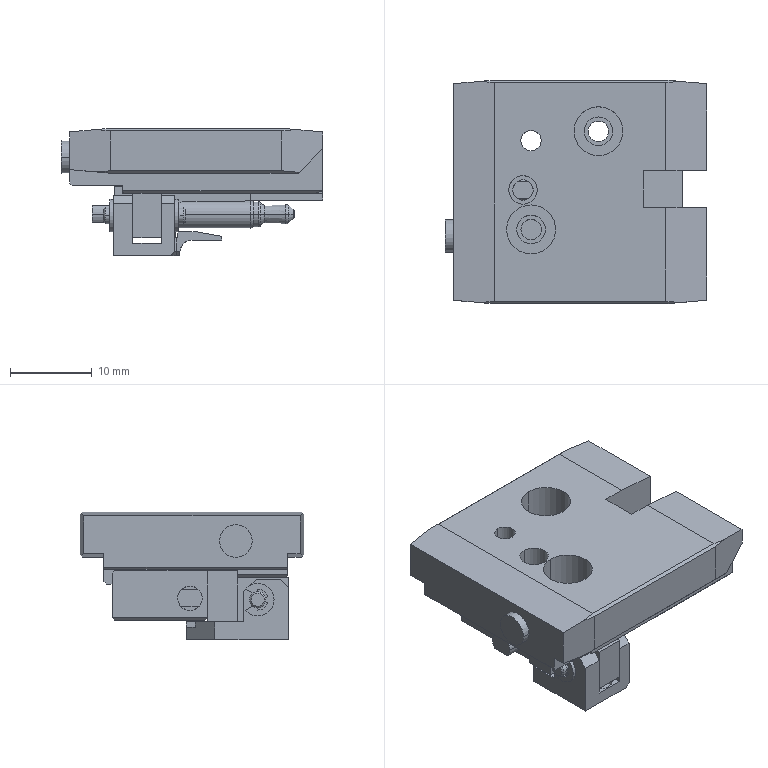Part | NX | 10 solids | 253 faces | box 32 x 27.4 x 15.605 mm | volume 6753 mm3 | plane 161 | cylinder 71 | cone 13 | torus 8 | commonest cylinder face diameters 2 x13 1.5 x10 2.5 x8 3.5 x8 3.1 x6 4 x6